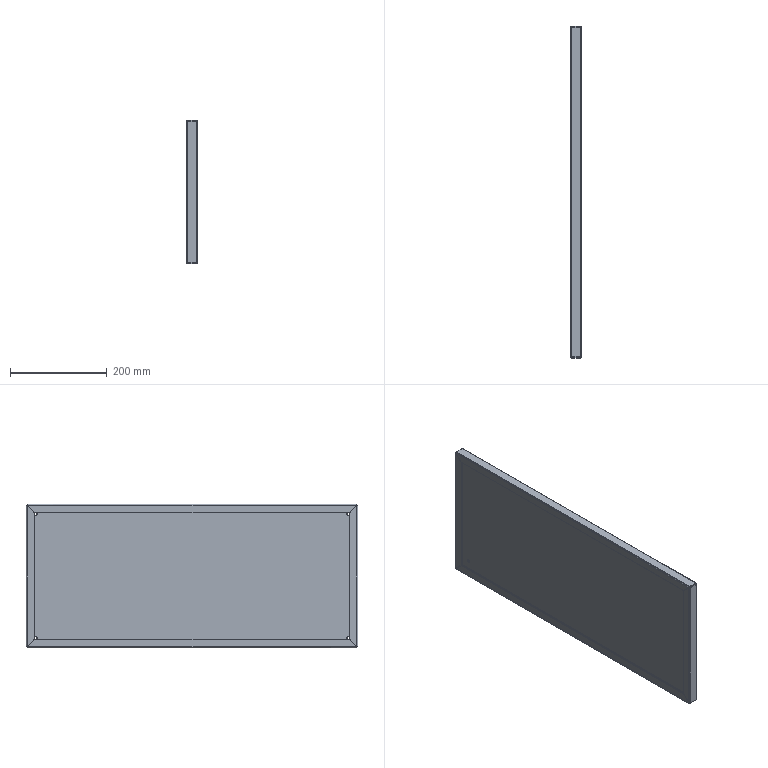Part | STEP file | PN_0074 front door | 1 solid | 78 faces | box 21.5 x 687 x 297 mm | volume 405902 mm3 | plane 38 | cylinder 24 | spline 16 | commonest cylinder face diameters 1.473 x8 4.473 x8 6 x8